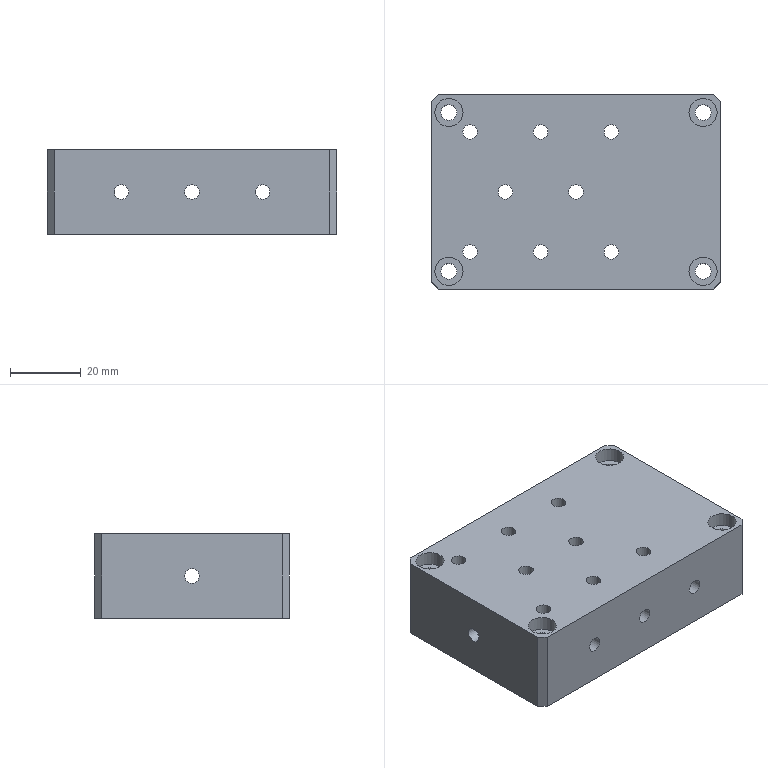NC program | NX | posted with a generic post | part box 82 x 55 x 24 mm
Whole program:
N10 G17 G21 G94 G90
(HOLE_MILLING_COPY , TOOL : D6)
N12 T12 M6
N14 G54
N16 G17 G0 G90 X0. Y0. B0. C0. S9500 M3
N18 G43 Z30. H12
N20 Z0.5
N22 G94 G3 X1.361 Y-1.361 R1.361 F1500.
N24 X2.723 Y0. R1.361
N26 X2.723 Y0. Z0. I-2.723 J0.
N28 X2.723 Y0. Z-0.5 I-2.723 J0.
N30 X2.723 Y0. Z-1. I-2.723 J0.
N32 X2.723 Y0. Z-1.5 I-2.723 J0.
N34 X2.723 Y0. Z-2. I-2.723 J0.
N36 X2.723 Y0. Z-2.5 I-2.723 J0.
N38 X2.723 Y0. Z-3. I-2.723 J0.
N40 X2.723 Y0. Z-3.5 I-2.723 J0.
N42 X2.723 Y0. Z-4. I-2.723 J0.
N44 X2.723 Y0. Z-4.5 I-2.723 J0.
N46 X2.723 Y0. Z-5. I-2.723 J0.
N48 X2.723 Y0. Z-5.5 I-2.723 J0.
N50 X2.723 Y0. Z-6. I-2.723 J0.
N52 X2.723 Y0. Z-6.5 I-2.723 J0.
N54 X2.723 Y0. Z-7. I-2.723 J0.
N56 X2.723 Y0. Z-7.5 I-2.723 J0.
N58 X2.723 Y0. Z-8. I-2.723 J0.
N60 X0. Y2.723 R2.723
N62 X2.723 Y0. R-2.723
N64 X1.361 Y1.361 R1.361
N66 X0. Y0. R1.361
N68 G0 Z30.
N70 M5
(PLANAR_MILL_COPY_COPY_COPY_COPY_1 , TOOL : D6A45)
N72 T01 M6
N74 G54
N76 G17 G0 G90 X1.443 Y3.323 B0. C0. S9500 M3
N78 G43 Z30. H1
N80 Z0.5
N82 G94 G1 Z-1. F1250.
N84 X0.866 Y4.323
N86 G3 X0. Y4.823 R1.
N88 X-4.823 Y0. R4.823
N90 X0. Y4.823 R-4.823
N92 X-0.866 Y4.323 R1.
N94 G1 X-1.443 Y3.323
N96 Z0.5
N98 G0 Z30.
N100 M5
N102 M2